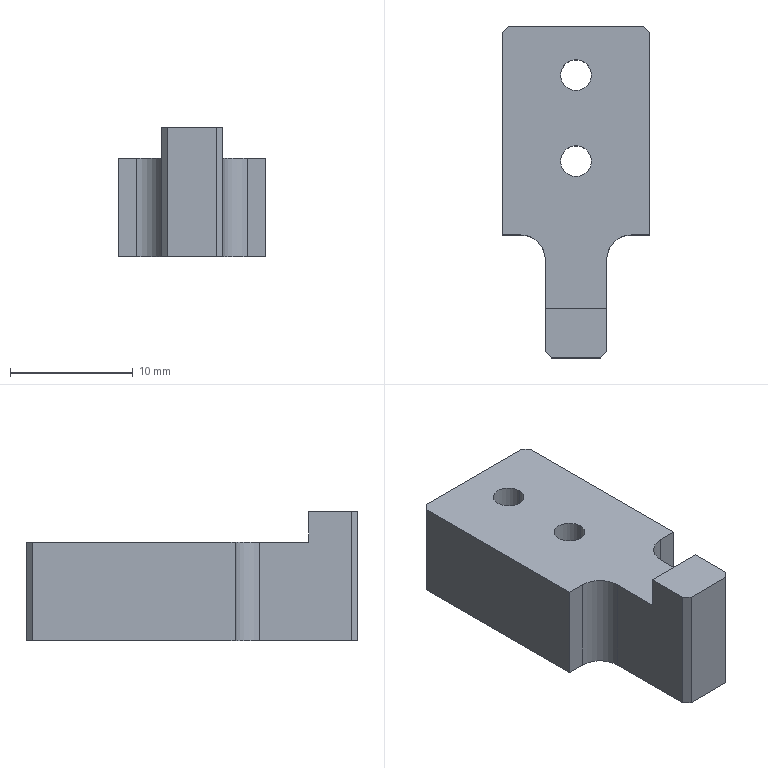Part | SolidWorks | features ICE 3, Chamfer 1, Extrusion 1, HoleWzd 1 | 1 solid | 29 faces | box 12 x 27 x 10.5 mm | volume 1656 mm3 | plane 20 | cylinder 9 | commonest cylinder face diameters 2.5 x4 1 x3 4 x2
STEP:
#1=CARTESIAN_POINT('',(1.25,23.,-2.5));
#2=VERTEX_POINT('',#1);
#3=CARTESIAN_POINT('',(-1.25,23.,-2.5));
#4=VERTEX_POINT('',#3);
#5=CARTESIAN_POINT('',(0.,23.,-2.5));
#6=DIRECTION('',(0.,0.,-1.));
#7=DIRECTION('',(-1.,0.,0.));
#8=AXIS2_PLACEMENT_3D('',#5,#6,#7);
#9=CIRCLE('',#8,1.25);
#10=EDGE_CURVE('',#2,#4,#9,.T.);
#11=ORIENTED_EDGE('',*,*,#10,.F.);
#12=CARTESIAN_POINT('',(1.25,23.,-7.3));
#13=VERTEX_POINT('',#12);
#14=CARTESIAN_POINT('',(1.25,23.,-7.3));
#15=DIRECTION('',(0.,0.,-1.));
#16=VECTOR('',#15,1000.);
#17=LINE('',#14,#16);
#18=EDGE_CURVE('',#2,#13,#17,.T.);
#19=ORIENTED_EDGE('',*,*,#18,.T.);
#20=CARTESIAN_POINT('',(-1.25,23.,-7.3));
#21=VERTEX_POINT('',#20);
#22=CARTESIAN_POINT('',(0.,23.,-7.3));
#23=DIRECTION('',(0.,0.,-1.));
#24=DIRECTION('',(-1.,0.,0.));
#25=AXIS2_PLACEMENT_3D('',#22,#23,#24);
#26=CIRCLE('',#25,1.25);
#27=EDGE_CURVE('',#13,#21,#26,.T.);
#28=ORIENTED_EDGE('',*,*,#27,.T.);
#29=CARTESIAN_POINT('',(-1.25,23.,-7.3));
#30=DIRECTION('',(0.,0.,-1.));
#31=VECTOR('',#30,1000.);
#32=LINE('',#29,#31);
#33=EDGE_CURVE('',#4,#21,#32,.T.);
#34=ORIENTED_EDGE('',*,*,#33,.F.);
#35=EDGE_LOOP('',(#11,#19,#28,#34));
#36=FACE_OUTER_BOUND('',#35,.T.);
#37=CARTESIAN_POINT('',(0.,23.,-7.3));
#38=DIRECTION('',(0.,0.,-1.));
#39=DIRECTION('',(-1.,0.,0.));
#40=AXIS2_PLACEMENT_3D('',#37,#38,#39);
#41=CYLINDRICAL_SURFACE('',#40,1.25);
#42=ADVANCED_FACE('',(#36),#41,.F.);
#43=CARTESIAN_POINT('',(1.25,16.,-2.5));
#44=VERTEX_POINT('',#43);
#45=CARTESIAN_POINT('',(-1.25,16.,-2.5));
#46=VERTEX_POINT('',#45);
#47=CARTESIAN_POINT('',(0.,16.,-2.5));
#48=DIRECTION('',(0.,0.,-1.));
#49=DIRECTION('',(-1.,0.,0.));
#50=AXIS2_PLACEMENT_3D('',#47,#48,#49);
#51=CIRCLE('',#50,1.25);
#52=EDGE_CURVE('',#44,#46,#51,.T.);
#53=ORIENTED_EDGE('',*,*,#52,.F.);
#54=CARTESIAN_POINT('',(1.25,16.,-7.3));
#55=VERTEX_POINT('',#54);
#56=CARTESIAN_POINT('',(1.25,16.,-7.3));
#57=DIRECTION('',(0.,0.,-1.));
#58=VECTOR('',#57,1000.);
#59=LINE('',#56,#58);
#60=EDGE_CURVE('',#44,#55,#59,.T.);
#61=ORIENTED_EDGE('',*,*,#60,.T.);
#62=CARTESIAN_POINT('',(-1.25,16.,-7.3));
#63=VERTEX_POINT('',#62);
#64=CARTESIAN_POINT('',(0.,16.,-7.3));
#65=DIRECTION('',(0.,0.,-1.));
#66=DIRECTION('',(-1.,0.,0.));
#67=AXIS2_PLACEMENT_3D('',#64,#65,#66);
#68=CIRCLE('',#67,1.25);
#69=EDGE_CURVE('',#55,#63,#68,.T.);
#70=ORIENTED_EDGE('',*,*,#69,.T.);
#71=CARTESIAN_POINT('',(-1.25,16.,-7.3));
#72=DIRECTION('',(0.,0.,-1.));
#73=VECTOR('',#72,1000.);
#74=LINE('',#71,#73);
#75=EDGE_CURVE('',#46,#63,#74,.T.);
#76=ORIENTED_EDGE('',*,*,#75,.F.);
#77=EDGE_LOOP('',(#53,#61,#70,#76));
#78=FACE_OUTER_BOUND('',#77,.T.);
#79=CARTESIAN_POINT('',(0.,16.,-7.3));
#80=DIRECTION('',(0.,0.,-1.));
#81=DIRECTION('',(-1.,0.,0.));
#82=AXIS2_PLACEMENT_3D('',#79,#80,#81);
#83=CYLINDRICAL_SURFACE('',#82,1.25);
#84=ADVANCED_FACE('',(#78),#83,.F.);
#85=CARTESIAN_POINT('',(-4.,12.5,-7.3));
#86=VERTEX_POINT('',#85);
#87=CARTESIAN_POINT('',(-4.5,12.,-7.3));
#88=VERTEX_POINT('',#87);
#89=CARTESIAN_POINT('',(-4.,12.,-7.3));
#90=DIRECTION('',(0.,0.,1.));
#91=DIRECTION('',(1.,0.,0.));
#92=AXIS2_PLACEMENT_3D('',#89,#90,#91);
#93=CIRCLE('',#92,0.5);
#94=EDGE_CURVE('',#86,#88,#93,.T.);
#95=ORIENTED_EDGE('',*,*,#94,.T.);
#96=CARTESIAN_POINT('',(-4.5,12.,-10.5));
#97=VERTEX_POINT('',#96);
#98=CARTESIAN_POINT('',(-4.5,12.,-7.3));
#99=DIRECTION('',(0.,0.,-1.));
#100=VECTOR('',#99,1000.);
#101=LINE('',#98,#100);
#102=EDGE_CURVE('',#88,#97,#101,.T.);
#103=ORIENTED_EDGE('',*,*,#102,.T.);
#104=CARTESIAN_POINT('',(-4.,12.5,-10.5));
#105=VERTEX_POINT('',#104);
#106=CARTESIAN_POINT('',(-4.,12.,-10.5));
#107=DIRECTION('',(0.,0.,1.));
#108=DIRECTION('',(1.,0.,0.));
#109=AXIS2_PLACEMENT_3D('',#106,#107,#108);
#110=CIRCLE('',#109,0.5);
#111=EDGE_CURVE('',#105,#97,#110,.T.);
#112=ORIENTED_EDGE('',*,*,#111,.F.);
#113=CARTESIAN_POINT('',(-4.,12.5,-7.3));
#114=DIRECTION('',(0.,0.,-1.));
#115=VECTOR('',#114,1000.);
#116=LINE('',#113,#115);
#117=EDGE_CURVE('',#86,#105,#116,.T.);
#118=ORIENTED_EDGE('',*,*,#117,.F.);
#119=EDGE_LOOP('',(#95,#103,#112,#118));
#120=FACE_OUTER_BOUND('',#119,.T.);
#121=CARTESIAN_POINT('',(-4.,12.,-7.3));
#122=DIRECTION('',(0.,0.,-1.));
#123=DIRECTION('',(-1.,0.,0.));
#124=AXIS2_PLACEMENT_3D('',#121,#122,#123);
#125=CYLINDRICAL_SURFACE('',#124,0.5);
#126=ADVANCED_FACE('',(#120),#125,.F.);
#127=CARTESIAN_POINT('',(2.,0.,-10.5));
#128=VERTEX_POINT('',#127);
#129=CARTESIAN_POINT('',(-2.,0.,-10.5));
#130=VERTEX_POINT('',#129);
#131=CARTESIAN_POINT('',(6.,0.,-10.5));
#132=DIRECTION('',(-1.,0.,0.));
#133=VECTOR('',#132,1000.);
#134=LINE('',#131,#133);
#135=EDGE_CURVE('',#128,#130,#134,.T.);
#136=ORIENTED_EDGE('',*,*,#135,.T.);
#137=CARTESIAN_POINT('',(-2.5,0.5,-10.5));
#138=VERTEX_POINT('',#137);
#139=CARTESIAN_POINT('',(-2.5,0.5,-10.5));
#140=DIRECTION('',(-0.7071,0.7071,0.));
#141=VECTOR('',#140,1000.);
#142=LINE('',#139,#141);
#143=EDGE_CURVE('',#130,#138,#142,.T.);
#144=ORIENTED_EDGE('',*,*,#143,.T.);
#145=CARTESIAN_POINT('',(-2.5,8.,-10.5));
#146=VERTEX_POINT('',#145);
#147=CARTESIAN_POINT('',(-2.5,0.,-10.5));
#148=DIRECTION('',(0.,1.,0.));
#149=VECTOR('',#148,1000.);
#150=LINE('',#147,#149);
#151=EDGE_CURVE('',#138,#146,#150,.T.);
#152=ORIENTED_EDGE('',*,*,#151,.T.);
#153=CARTESIAN_POINT('',(-4.5,10.,-10.5));
#154=VERTEX_POINT('',#153);
#155=CARTESIAN_POINT('',(-4.5,8.,-10.5));
#156=DIRECTION('',(0.,0.,1.));
#157=DIRECTION('',(1.,0.,0.));
#158=AXIS2_PLACEMENT_3D('',#155,#156,#157);
#159=CIRCLE('',#158,2.);
#160=EDGE_CURVE('',#146,#154,#159,.T.);
#161=ORIENTED_EDGE('',*,*,#160,.T.);
#162=CARTESIAN_POINT('',(-6.,10.,-10.5));
#163=VERTEX_POINT('',#162);
#164=CARTESIAN_POINT('',(-6.,10.,-10.5));
#165=DIRECTION('',(-1.,0.,0.));
#166=VECTOR('',#165,1000.);
#167=LINE('',#164,#166);
#168=EDGE_CURVE('',#154,#163,#167,.T.);
#169=ORIENTED_EDGE('',*,*,#168,.T.);
#170=CARTESIAN_POINT('',(-6.,26.5,-10.5));
#171=VERTEX_POINT('',#170);
#172=CARTESIAN_POINT('',(-6.,27.,-10.5));
#173=DIRECTION('',(0.,1.,0.));
#174=VECTOR('',#173,1000.);
#175=LINE('',#172,#174);
#176=EDGE_CURVE('',#163,#171,#175,.T.);
#177=ORIENTED_EDGE('',*,*,#176,.T.);
#178=CARTESIAN_POINT('',(-5.5,27.,-10.5));
#179=VERTEX_POINT('',#178);
#180=CARTESIAN_POINT('',(-5.5,27.,-10.5));
#181=DIRECTION('',(0.7071,0.7071,0.));
#182=VECTOR('',#181,1000.);
#183=LINE('',#180,#182);
#184=EDGE_CURVE('',#171,#179,#183,.T.);
#185=ORIENTED_EDGE('',*,*,#184,.T.);
#186=CARTESIAN_POINT('',(-4.,27.,-10.5));
#187=VERTEX_POINT('',#186);
#188=CARTESIAN_POINT('',(6.,27.,-10.5));
#189=DIRECTION('',(-1.,0.,0.));
#190=VECTOR('',#189,1000.);
#191=LINE('',#188,#190);
#192=EDGE_CURVE('',#187,#179,#191,.T.);
#193=ORIENTED_EDGE('',*,*,#192,.F.);
#194=CARTESIAN_POINT('',(-4.,27.,-10.5));
#195=DIRECTION('',(0.,-1.,0.));
#196=VECTOR('',#195,1000.);
#197=LINE('',#194,#196);
#198=EDGE_CURVE('',#187,#105,#197,.T.);
#199=ORIENTED_EDGE('',*,*,#198,.T.);
#200=ORIENTED_EDGE('',*,*,#111,.T.);
#201=CARTESIAN_POINT('',(-3.5,12.,-10.5));
#202=VERTEX_POINT('',#201);
#203=CARTESIAN_POINT('',(-4.,12.,-10.5));
#204=DIRECTION('',(0.,0.,1.));
#205=DIRECTION('',(1.,0.,0.));
#206=AXIS2_PLACEMENT_3D('',#203,#204,#205);
#207=CIRCLE('',#206,0.5);
#208=EDGE_CURVE('',#97,#202,#207,.T.);
#209=ORIENTED_EDGE('',*,*,#208,.T.);
#210=CARTESIAN_POINT('',(3.5,12.,-10.5));
#211=VERTEX_POINT('',#210);
#212=CARTESIAN_POINT('',(-3.5,12.,-10.5));
#213=DIRECTION('',(1.,0.,0.));
#214=VECTOR('',#213,1000.);
#215=LINE('',#212,#214);
#216=EDGE_CURVE('',#202,#211,#215,.T.);
#217=ORIENTED_EDGE('',*,*,#216,.T.);
#218=CARTESIAN_POINT('',(4.,12.5,-10.5));
#219=VERTEX_POINT('',#218);
#220=CARTESIAN_POINT('',(4.,12.,-10.5));
#221=DIRECTION('',(0.,0.,1.));
#222=DIRECTION('',(1.,0.,0.));
#223=AXIS2_PLACEMENT_3D('',#220,#221,#222);
#224=CIRCLE('',#223,0.5);
#225=EDGE_CURVE('',#211,#219,#224,.T.);
#226=ORIENTED_EDGE('',*,*,#225,.T.);
#227=CARTESIAN_POINT('',(4.,27.,-10.5));
#228=VERTEX_POINT('',#227);
#229=CARTESIAN_POINT('',(4.,27.,-10.5));
#230=DIRECTION('',(0.,1.,0.));
#231=VECTOR('',#230,1000.);
#232=LINE('',#229,#231);
#233=EDGE_CURVE('',#219,#228,#232,.T.);
#234=ORIENTED_EDGE('',*,*,#233,.T.);
#235=CARTESIAN_POINT('',(5.5,27.,-10.5));
#236=VERTEX_POINT('',#235);
#237=CARTESIAN_POINT('',(6.,27.,-10.5));
#238=DIRECTION('',(-1.,0.,0.));
#239=VECTOR('',#238,1000.);
#240=LINE('',#237,#239);
#241=EDGE_CURVE('',#236,#228,#240,.T.);
#242=ORIENTED_EDGE('',*,*,#241,.F.);
#243=CARTESIAN_POINT('',(6.,26.5,-10.5));
#244=VERTEX_POINT('',#243);
#245=CARTESIAN_POINT('',(6.,26.5,-10.5));
#246=DIRECTION('',(0.7071,-0.7071,0.));
#247=VECTOR('',#246,1000.);
#248=LINE('',#245,#247);
#249=EDGE_CURVE('',#236,#244,#248,.T.);
#250=ORIENTED_EDGE('',*,*,#249,.T.);
#251=CARTESIAN_POINT('',(6.,10.,-10.5));
#252=VERTEX_POINT('',#251);
#253=CARTESIAN_POINT('',(6.,27.,-10.5));
#254=DIRECTION('',(0.,1.,0.));
#255=VECTOR('',#254,1000.);
#256=LINE('',#253,#255);
#257=EDGE_CURVE('',#252,#244,#256,.T.);
#258=ORIENTED_EDGE('',*,*,#257,.F.);
#259=CARTESIAN_POINT('',(4.5,10.,-10.5));
#260=VERTEX_POINT('',#259);
#261=CARTESIAN_POINT('',(6.,10.,-10.5));
#262=DIRECTION('',(-1.,0.,0.));
#263=VECTOR('',#262,1000.);
#264=LINE('',#261,#263);
#265=EDGE_CURVE('',#252,#260,#264,.T.);
#266=ORIENTED_EDGE('',*,*,#265,.T.);
#267=CARTESIAN_POINT('',(2.5,8.,-10.5));
#268=VERTEX_POINT('',#267);
#269=CARTESIAN_POINT('',(4.5,8.,-10.5));
#270=DIRECTION('',(0.,0.,1.));
#271=DIRECTION('',(1.,0.,0.));
#272=AXIS2_PLACEMENT_3D('',#269,#270,#271);
#273=CIRCLE('',#272,2.);
#274=EDGE_CURVE('',#260,#268,#273,.T.);
#275=ORIENTED_EDGE('',*,*,#274,.T.);
#276=CARTESIAN_POINT('',(2.5,0.5,-10.5));
#277=VERTEX_POINT('',#276);
#278=CARTESIAN_POINT('',(2.5,0.,-10.5));
#279=DIRECTION('',(0.,-1.,0.));
#280=VECTOR('',#279,1000.);
#281=LINE('',#278,#280);
#282=EDGE_CURVE('',#268,#277,#281,.T.);
#283=ORIENTED_EDGE('',*,*,#282,.T.);
#284=CARTESIAN_POINT('',(2.,0.,-10.5));
#285=DIRECTION('',(-0.7071,-0.7071,0.));
#286=VECTOR('',#285,1000.);
#287=LINE('',#284,#286);
#288=EDGE_CURVE('',#277,#128,#287,.T.);
#289=ORIENTED_EDGE('',*,*,#288,.T.);
#290=EDGE_LOOP('',(#136,#144,#152,#161,#169,#177,#185,#193,#199,#200,#209,#217,#226,#234,#242,#250,#258,#266,#275,#283,#289));
#291=FACE_OUTER_BOUND('',#290,.T.);
#292=CARTESIAN_POINT('',(6.,27.,-10.5));
#293=DIRECTION('',(0.,0.,1.));
#294=DIRECTION('',(0.,-1.,0.));
#295=AXIS2_PLACEMENT_3D('',#292,#293,#294);
#296=PLANE('',#295);
#297=ADVANCED_FACE('',(#291),#296,.F.);
#298=ORIENTED_EDGE('',*,*,#192,.T.);
#299=CARTESIAN_POINT('',(-5.5,27.,-2.5));
#300=VERTEX_POINT('',#299);
#301=CARTESIAN_POINT('',(-5.5,27.,-2.5));
#302=DIRECTION('',(0.,0.,1.));
#303=VECTOR('',#302,1000.);
#304=LINE('',#301,#303);
#305=EDGE_CURVE('',#179,#300,#304,.T.);
#306=ORIENTED_EDGE('',*,*,#305,.T.);
#307=CARTESIAN_POINT('',(5.5,27.,-2.5));
#308=VERTEX_POINT('',#307);
#309=CARTESIAN_POINT('',(6.,27.,-2.5));
#310=DIRECTION('',(-1.,0.,0.));
#311=VECTOR('',#310,1000.);
#312=LINE('',#309,#311);
#313=EDGE_CURVE('',#308,#300,#312,.T.);
#314=ORIENTED_EDGE('',*,*,#313,.F.);
#315=CARTESIAN_POINT('',(5.5,27.,-10.5));
#316=DIRECTION('',(0.,0.,-1.));
#317=VECTOR('',#316,1000.);
#318=LINE('',#315,#317);
#319=EDGE_CURVE('',#308,#236,#318,.T.);
#320=ORIENTED_EDGE('',*,*,#319,.T.);
#321=ORIENTED_EDGE('',*,*,#241,.T.);
#322=CARTESIAN_POINT('',(4.,27.,-7.3));
#323=VERTEX_POINT('',#322);
#324=CARTESIAN_POINT('',(4.,27.,-7.3));
#325=DIRECTION('',(0.,0.,-1.));
#326=VECTOR('',#325,1000.);
#327=LINE('',#324,#326);
#328=EDGE_CURVE('',#323,#228,#327,.T.);
#329=ORIENTED_EDGE('',*,*,#328,.F.);
#330=CARTESIAN_POINT('',(-4.,27.,-7.3));
#331=VERTEX_POINT('',#330);
#332=CARTESIAN_POINT('',(-4.,27.,-7.3));
#333=DIRECTION('',(-1.,0.,0.));
#334=VECTOR('',#333,1000.);
#335=LINE('',#332,#334);
#336=EDGE_CURVE('',#323,#331,#335,.T.);
#337=ORIENTED_EDGE('',*,*,#336,.T.);
#338=CARTESIAN_POINT('',(-4.,27.,-7.3));
#339=DIRECTION('',(0.,0.,-1.));
#340=VECTOR('',#339,1000.);
#341=LINE('',#338,#340);
#342=EDGE_CURVE('',#331,#187,#341,.T.);
#343=ORIENTED_EDGE('',*,*,#342,.T.);
#344=EDGE_LOOP('',(#298,#306,#314,#320,#321,#329,#337,#343));
#345=FACE_OUTER_BOUND('',#344,.T.);
#346=CARTESIAN_POINT('',(6.,27.,-2.5));
#347=DIRECTION('',(0.,-1.,0.));
#348=DIRECTION('',(0.,0.,-1.));
#349=AXIS2_PLACEMENT_3D('',#346,#347,#348);
#350=PLANE('',#349);
#351=ADVANCED_FACE('',(#345),#350,.F.);
#352=CARTESIAN_POINT('',(2.5,4.,0.));
#353=VERTEX_POINT('',#352);
#354=CARTESIAN_POINT('',(-2.5,4.,0.));
#355=VERTEX_POINT('',#354);
#356=CARTESIAN_POINT('',(6.,4.,0.));
#357=DIRECTION('',(-1.,0.,0.));
#358=VECTOR('',#357,1000.);
#359=LINE('',#356,#358);
#360=EDGE_CURVE('',#353,#355,#359,.T.);
#361=ORIENTED_EDGE('',*,*,#360,.F.);
#362=CARTESIAN_POINT('',(2.5,4.,-2.5));
#363=VERTEX_POINT('',#362);
#364=CARTESIAN_POINT('',(2.5,4.,-2.5));
#365=DIRECTION('',(0.,0.,-1.));
#366=VECTOR('',#365,1000.);
#367=LINE('',#364,#366);
#368=EDGE_CURVE('',#353,#363,#367,.T.);
#369=ORIENTED_EDGE('',*,*,#368,.T.);
#370=CARTESIAN_POINT('',(-2.5,4.,-2.5));
#371=VERTEX_POINT('',#370);
#372=CARTESIAN_POINT('',(6.,4.,-2.5));
#373=DIRECTION('',(-1.,0.,0.));
#374=VECTOR('',#373,1000.);
#375=LINE('',#372,#374);
#376=EDGE_CURVE('',#363,#371,#375,.T.);
#377=ORIENTED_EDGE('',*,*,#376,.T.);
#378=CARTESIAN_POINT('',(-2.5,4.,-2.5));
#379=DIRECTION('',(0.,0.,1.));
#380=VECTOR('',#379,1000.);
#381=LINE('',#378,#380);
#382=EDGE_CURVE('',#371,#355,#381,.T.);
#383=ORIENTED_EDGE('',*,*,#382,.T.);
#384=EDGE_LOOP('',(#361,#369,#377,#383));
#385=FACE_OUTER_BOUND('',#384,.T.);
#386=CARTESIAN_POINT('',(6.,4.,-2.5));
#387=DIRECTION('',(0.,-1.,0.));
#388=DIRECTION('',(0.,0.,-1.));
#389=AXIS2_PLACEMENT_3D('',#386,#387,#388);
#390=PLANE('',#389);
#391=ADVANCED_FACE('',(#385),#390,.F.);
#392=CARTESIAN_POINT('',(-2.5,0.5,0.));
#393=VERTEX_POINT('',#392);
#394=CARTESIAN_POINT('',(-2.5,0.,0.));
#395=DIRECTION('',(0.,1.,0.));
#396=VECTOR('',#395,1000.);
#397=LINE('',#394,#396);
#398=EDGE_CURVE('',#393,#355,#397,.T.);
#399=ORIENTED_EDGE('',*,*,#398,.F.);
#400=CARTESIAN_POINT('',(-2.,0.,0.));
#401=VERTEX_POINT('',#400);
#402=CARTESIAN_POINT('',(-2.5,0.5,0.));
#403=DIRECTION('',(0.7071,-0.7071,0.));
#404=VECTOR('',#403,1000.);
#405=LINE('',#402,#404);
#406=EDGE_CURVE('',#393,#401,#405,.T.);
#407=ORIENTED_EDGE('',*,*,#406,.T.);
#408=CARTESIAN_POINT('',(2.,0.,0.));
#409=VERTEX_POINT('',#408);
#410=CARTESIAN_POINT('',(6.,0.,0.));
#411=DIRECTION('',(-1.,0.,0.));
#412=VECTOR('',#411,1000.);
#413=LINE('',#410,#412);
#414=EDGE_CURVE('',#409,#401,#413,.T.);
#415=ORIENTED_EDGE('',*,*,#414,.F.);
#416=CARTESIAN_POINT('',(2.5,0.5,0.));
#417=VERTEX_POINT('',#416);
#418=CARTESIAN_POINT('',(2.,0.,0.));
#419=DIRECTION('',(0.7071,0.7071,0.));
#420=VECTOR('',#419,1000.);
#421=LINE('',#418,#420);
#422=EDGE_CURVE('',#409,#417,#421,.T.);
#423=ORIENTED_EDGE('',*,*,#422,.T.);
#424=CARTESIAN_POINT('',(2.5,0.,0.));
#425=DIRECTION('',(0.,-1.,0.));
#426=VECTOR('',#425,1000.);
#427=LINE('',#424,#426);
#428=EDGE_CURVE('',#353,#417,#427,.T.);
#429=ORIENTED_EDGE('',*,*,#428,.F.);
#430=ORIENTED_EDGE('',*,*,#360,.T.);
#431=EDGE_LOOP('',(#399,#407,#415,#423,#429,#430));
#432=FACE_OUTER_BOUND('',#431,.T.);
#433=CARTESIAN_POINT('',(6.,4.,0.));
#434=DIRECTION('',(0.,0.,-1.));
#435=DIRECTION('',(-1.,0.,0.));
#436=AXIS2_PLACEMENT_3D('',#433,#434,#435);
#437=PLANE('',#436);
#438=ADVANCED_FACE('',(#432),#437,.F.);
#439=ORIENTED_EDGE('',*,*,#414,.T.);
#440=CARTESIAN_POINT('',(-2.,0.,-10.5));
#441=DIRECTION('',(0.,0.,-1.));
#442=VECTOR('',#441,1000.);
#443=LINE('',#440,#442);
#444=EDGE_CURVE('',#401,#130,#443,.T.);
#445=ORIENTED_EDGE('',*,*,#444,.T.);
#446=ORIENTED_EDGE('',*,*,#135,.F.);
#447=CARTESIAN_POINT('',(2.,0.,-10.5));
#448=DIRECTION('',(0.,0.,1.));
#449=VECTOR('',#448,1000.);
#450=LINE('',#447,#449);
#451=EDGE_CURVE('',#128,#409,#450,.T.);
#452=ORIENTED_EDGE('',*,*,#451,.T.);
#453=EDGE_LOOP('',(#439,#445,#446,#452));
#454=FACE_OUTER_BOUND('',#453,.T.);
#455=CARTESIAN_POINT('',(6.,0.,-10.5));
#456=DIRECTION('',(0.,1.,0.));
#457=DIRECTION('',(0.,0.,1.));
#458=AXIS2_PLACEMENT_3D('',#455,#456,#457);
#459=PLANE('',#458);
#460=ADVANCED_FACE('',(#454),#459,.F.);
#461=CARTESIAN_POINT('',(0.,23.,-2.5));
#462=DIRECTION('',(0.,0.,-1.));
#463=DIRECTION('',(-1.,0.,0.));
#464=AXIS2_PLACEMENT_3D('',#461,#462,#463);
#465=CIRCLE('',#464,1.25);
#466=EDGE_CURVE('',#4,#2,#465,.T.);
#467=ORIENTED_EDGE('',*,*,#466,.T.);
#468=ORIENTED_EDGE('',*,*,#10,.T.);
#469=EDGE_LOOP('',(#467,#468));
#470=FACE_BOUND('',#469,.T.);
#471=CARTESIAN_POINT('',(0.,16.,-2.5));
#472=DIRECTION('',(0.,0.,-1.));
#473=DIRECTION('',(-1.,0.,0.));
#474=AXIS2_PLACEMENT_3D('',#471,#472,#473);
#475=CIRCLE('',#474,1.25);
#476=EDGE_CURVE('',#46,#44,#475,.T.);
#477=ORIENTED_EDGE('',*,*,#476,.T.);
#478=ORIENTED_EDGE('',*,*,#52,.T.);
#479=EDGE_LOOP('',(#477,#478));
#480=FACE_BOUND('',#479,.T.);
#481=ORIENTED_EDGE('',*,*,#313,.T.);
#482=CARTESIAN_POINT('',(-6.,26.5,-2.5));
#483=VERTEX_POINT('',#482);
#484=CARTESIAN_POINT('',(-5.5,27.,-2.5));
#485=DIRECTION('',(-0.7071,-0.7071,0.));
#486=VECTOR('',#485,1000.);
#487=LINE('',#484,#486);
#488=EDGE_CURVE('',#300,#483,#487,.T.);
#489=ORIENTED_EDGE('',*,*,#488,.T.);
#490=CARTESIAN_POINT('',(-6.,10.,-2.5));
#491=VERTEX_POINT('',#490);
#492=CARTESIAN_POINT('',(-6.,4.,-2.5));
#493=DIRECTION('',(0.,-1.,0.));
#494=VECTOR('',#493,1000.);
#495=LINE('',#492,#494);
#496=EDGE_CURVE('',#483,#491,#495,.T.);
#497=ORIENTED_EDGE('',*,*,#496,.T.);
#498=CARTESIAN_POINT('',(-4.5,10.,-2.5));
#499=VERTEX_POINT('',#498);
#500=CARTESIAN_POINT('',(6.,10.,-2.5));
#501=DIRECTION('',(1.,0.,0.));
#502=VECTOR('',#501,1000.);
#503=LINE('',#500,#502);
#504=EDGE_CURVE('',#491,#499,#503,.T.);
#505=ORIENTED_EDGE('',*,*,#504,.T.);
#506=CARTESIAN_POINT('',(-2.5,8.,-2.5));
#507=VERTEX_POINT('',#506);
#508=CARTESIAN_POINT('',(-4.5,8.,-2.5));
#509=DIRECTION('',(0.,0.,-1.));
#510=DIRECTION('',(-1.,0.,0.));
#511=AXIS2_PLACEMENT_3D('',#508,#509,#510);
#512=CIRCLE('',#511,2.);
#513=EDGE_CURVE('',#499,#507,#512,.T.);
#514=ORIENTED_EDGE('',*,*,#513,.T.);
#515=CARTESIAN_POINT('',(-2.5,4.,-2.5));
#516=DIRECTION('',(0.,-1.,0.));
#517=VECTOR('',#516,1000.);
#518=LINE('',#515,#517);
#519=EDGE_CURVE('',#507,#371,#518,.T.);
#520=ORIENTED_EDGE('',*,*,#519,.T.);
#521=ORIENTED_EDGE('',*,*,#376,.F.);
#522=CARTESIAN_POINT('',(2.5,8.,-2.5));
#523=VERTEX_POINT('',#522);
#524=CARTESIAN_POINT('',(2.5,4.,-2.5));
#525=DIRECTION('',(0.,1.,0.));
#526=VECTOR('',#525,1000.);
#527=LINE('',#524,#526);
#528=EDGE_CURVE('',#363,#523,#527,.T.);
#529=ORIENTED_EDGE('',*,*,#528,.T.);
#530=CARTESIAN_POINT('',(4.5,10.,-2.5));
#531=VERTEX_POINT('',#530);
#532=CARTESIAN_POINT('',(4.5,8.,-2.5));
#533=DIRECTION('',(0.,0.,-1.));
#534=DIRECTION('',(-1.,0.,0.));
#535=AXIS2_PLACEMENT_3D('',#532,#533,#534);
#536=CIRCLE('',#535,2.);
#537=EDGE_CURVE('',#523,#531,#536,.T.);
#538=ORIENTED_EDGE('',*,*,#537,.T.);
#539=CARTESIAN_POINT('',(6.,10.,-2.5));
#540=VERTEX_POINT('',#539);
#541=CARTESIAN_POINT('',(6.,10.,-2.5));
#542=DIRECTION('',(1.,0.,0.));
#543=VECTOR('',#542,1000.);
#544=LINE('',#541,#543);
#545=EDGE_CURVE('',#531,#540,#544,.T.);
#546=ORIENTED_EDGE('',*,*,#545,.T.);
#547=CARTESIAN_POINT('',(6.,26.5,-2.5));
#548=VERTEX_POINT('',#547);
#549=CARTESIAN_POINT('',(6.,4.,-2.5));
#550=DIRECTION('',(0.,-1.,0.));
#551=VECTOR('',#550,1000.);
#552=LINE('',#549,#551);
#553=EDGE_CURVE('',#548,#540,#552,.T.);
#554=ORIENTED_EDGE('',*,*,#553,.F.);
#555=CARTESIAN_POINT('',(6.,26.5,-2.5));
#556=DIRECTION('',(-0.7071,0.7071,0.));
#557=VECTOR('',#556,1000.);
#558=LINE('',#555,#557);
#559=EDGE_CURVE('',#548,#308,#558,.T.);
#560=ORIENTED_EDGE('',*,*,#559,.T.);
#561=EDGE_LOOP('',(#481,#489,#497,#505,#514,#520,#521,#529,#538,#546,#554,#560));
#562=FACE_OUTER_BOUND('',#561,.T.);
#563=CARTESIAN_POINT('',(6.,4.,-2.5));
#564=DIRECTION('',(0.,0.,-1.));
#565=DIRECTION('',(-1.,0.,0.));
#566=AXIS2_PLACEMENT_3D('',#563,#564,#565);
#567=PLANE('',#566);
#568=ADVANCED_FACE('',(#470,#480,#562),#567,.F.);
#569=ORIENTED_EDGE('',*,*,#257,.T.);
#570=CARTESIAN_POINT('',(6.,26.5,-2.5));
#571=DIRECTION('',(0.,0.,1.));
#572=VECTOR('',#571,1000.);
#573=LINE('',#570,#572);
#574=EDGE_CURVE('',#244,#548,#573,.T.);
#575=ORIENTED_EDGE('',*,*,#574,.T.);
#576=ORIENTED_EDGE('',*,*,#553,.T.);
#577=CARTESIAN_POINT('',(6.,10.,-10.5));
#578=DIRECTION('',(0.,0.,1.));
#579=VECTOR('',#578,1000.);
#580=LINE('',#577,#579);
#581=EDGE_CURVE('',#252,#540,#580,.T.);
#582=ORIENTED_EDGE('',*,*,#581,.F.);
#583=EDGE_LOOP('',(#569,#575,#576,#582));
#584=FACE_OUTER_BOUND('',#583,.T.);
#585=CARTESIAN_POINT('',(6.,0.,0.));
#586=DIRECTION('',(1.,0.,0.));
#587=DIRECTION('',(0.,0.,-1.));
#588=AXIS2_PLACEMENT_3D('',#585,#586,#587);
#589=PLANE('',#588);
#590=ADVANCED_FACE('',(#584),#589,.T.);
#591=ORIENTED_EDGE('',*,*,#496,.F.);
#592=CARTESIAN_POINT('',(-6.,26.5,0.));
#593=DIRECTION('',(0.,0.,-1.));
#594=VECTOR('',#593,1000.);
#595=LINE('',#592,#594);
#596=EDGE_CURVE('',#483,#171,#595,.T.);
#597=ORIENTED_EDGE('',*,*,#596,.T.);
#598=ORIENTED_EDGE('',*,*,#176,.F.);
#599=CARTESIAN_POINT('',(-6.,10.,-10.5));
#600=DIRECTION('',(0.,0.,1.));
#601=VECTOR('',#600,1000.);
#602=LINE('',#599,#601);
#603=EDGE_CURVE('',#163,#491,#602,.T.);
#604=ORIENTED_EDGE('',*,*,#603,.T.);
#605=EDGE_LOOP('',(#591,#597,#598,#604));
#606=FACE_OUTER_BOUND('',#605,.T.);
#607=CARTESIAN_POINT('',(-6.,0.,0.));
#608=DIRECTION('',(1.,0.,0.));
#609=DIRECTION('',(0.,0.,-1.));
#610=AXIS2_PLACEMENT_3D('',#607,#608,#609);
#611=PLANE('',#610);
#612=ADVANCED_FACE('',(#606),#611,.F.);
#613=ORIENTED_EDGE('',*,*,#198,.F.);
#614=ORIENTED_EDGE('',*,*,#342,.F.);
#615=CARTESIAN_POINT('',(-4.,27.,-7.3));
#616=DIRECTION('',(0.,-1.,0.));
#617=VECTOR('',#616,1000.);
#618=LINE('',#615,#617);
#619=EDGE_CURVE('',#331,#86,#618,.T.);
#620=ORIENTED_EDGE('',*,*,#619,.T.);
#621=ORIENTED_EDGE('',*,*,#117,.T.);
#622=EDGE_LOOP('',(#613,#614,#620,#621));
#623=FACE_OUTER_BOUND('',#622,.T.);
#624=CARTESIAN_POINT('',(-4.,27.,-7.3));
#625=DIRECTION('',(1.,0.,0.));
#626=DIRECTION('',(0.,1.,0.));
#627=AXIS2_PLACEMENT_3D('',#624,#625,#626);
#628=PLANE('',#627);
#629=ADVANCED_FACE('',(#623),#628,.T.);
#630=ORIENTED_EDGE('',*,*,#102,.F.);
#631=CARTESIAN_POINT('',(-3.5,12.,-7.3));
#632=VERTEX_POINT('',#631);
#633=CARTESIAN_POINT('',(-4.,12.,-7.3));
#634=DIRECTION('',(0.,0.,1.));
#635=DIRECTION('',(1.,0.,0.));
#636=AXIS2_PLACEMENT_3D('',#633,#634,#635);
#637=CIRCLE('',#636,0.5);
#638=EDGE_CURVE('',#88,#632,#637,.T.);
#639=ORIENTED_EDGE('',*,*,#638,.T.);
#640=CARTESIAN_POINT('',(-3.5,12.,-7.3));
#641=DIRECTION('',(0.,0.,-1.));
#642=VECTOR('',#641,1000.);
#643=LINE('',#640,#642);
#644=EDGE_CURVE('',#632,#202,#643,.T.);
#645=ORIENTED_EDGE('',*,*,#644,.T.);
#646=ORIENTED_EDGE('',*,*,#208,.F.);
#647=EDGE_LOOP('',(#630,#639,#645,#646));
#648=FACE_OUTER_BOUND('',#647,.T.);
#649=CARTESIAN_POINT('',(-4.,12.,-7.3));
#650=DIRECTION('',(0.,0.,-1.));
#651=DIRECTION('',(-1.,0.,0.));
#652=AXIS2_PLACEMENT_3D('',#649,#650,#651);
#653=CYLINDRICAL_SURFACE('',#652,0.5);
#654=ADVANCED_FACE('',(#648),#653,.F.);
#655=ORIENTED_EDGE('',*,*,#216,.F.);
#656=ORIENTED_EDGE('',*,*,#644,.F.);
#657=CARTESIAN_POINT('',(3.5,12.,-7.3));
#658=VERTEX_POINT('',#657);
#659=CARTESIAN_POINT('',(-3.5,12.,-7.3));
#660=DIRECTION('',(1.,0.,0.));
#661=VECTOR('',#660,1000.);
#662=LINE('',#659,#661);
#663=EDGE_CURVE('',#632,#658,#662,.T.);
#664=ORIENTED_EDGE('',*,*,#663,.T.);
#665=CARTESIAN_POINT('',(3.5,12.,-7.3));
#666=DIRECTION('',(0.,0.,-1.));
#667=VECTOR('',#666,1000.);
#668=LINE('',#665,#667);
#669=EDGE_CURVE('',#658,#211,#668,.T.);
#670=ORIENTED_EDGE('',*,*,#669,.T.);
#671=EDGE_LOOP('',(#655,#656,#664,#670));
#672=FACE_OUTER_BOUND('',#671,.T.);
#673=CARTESIAN_POINT('',(-3.5,12.,-7.3));
#674=DIRECTION('',(0.,1.,0.));
#675=DIRECTION('',(0.,0.,1.));
#676=AXIS2_PLACEMENT_3D('',#673,#674,#675);
#677=PLANE('',#676);
#678=ADVANCED_FACE('',(#672),#677,.T.);
#679=ORIENTED_EDGE('',*,*,#225,.F.);
#680=ORIENTED_EDGE('',*,*,#669,.F.);
#681=CARTESIAN_POINT('',(4.,12.5,-7.3));
#682=VERTEX_POINT('',#681);
#683=CARTESIAN_POINT('',(4.,12.,-7.3));
#684=DIRECTION('',(0.,0.,1.));
#685=DIRECTION('',(1.,0.,0.));
#686=AXIS2_PLACEMENT_3D('',#683,#684,#685);
#687=CIRCLE('',#686,0.5);
#688=EDGE_CURVE('',#658,#682,#687,.T.);
#689=ORIENTED_EDGE('',*,*,#688,.T.);
#690=CARTESIAN_POINT('',(4.,12.5,-7.3));
#691=DIRECTION('',(0.,0.,-1.));
#692=VECTOR('',#691,1000.);
#693=LINE('',#690,#692);
#694=EDGE_CURVE('',#682,#219,#693,.T.);
#695=ORIENTED_EDGE('',*,*,#694,.T.);
#696=EDGE_LOOP('',(#679,#680,#689,#695));
#697=FACE_OUTER_BOUND('',#696,.T.);
#698=CARTESIAN_POINT('',(4.,12.,-7.3));
#699=DIRECTION('',(0.,0.,-1.));
#700=DIRECTION('',(-1.,0.,0.));
#701=AXIS2_PLACEMENT_3D('',#698,#699,#700);
#702=CYLINDRICAL_SURFACE('',#701,0.5);
#703=ADVANCED_FACE('',(#697),#702,.F.);
#704=ORIENTED_EDGE('',*,*,#233,.F.);
#705=ORIENTED_EDGE('',*,*,#694,.F.);
#706=CARTESIAN_POINT('',(4.,27.,-7.3));
#707=DIRECTION('',(0.,1.,0.));
#708=VECTOR('',#707,1000.);
#709=LINE('',#706,#708);
#710=EDGE_CURVE('',#682,#323,#709,.T.);
#711=ORIENTED_EDGE('',*,*,#710,.T.);
#712=ORIENTED_EDGE('',*,*,#328,.T.);
#713=EDGE_LOOP('',(#704,#705,#711,#712));
#714=FACE_OUTER_BOUND('',#713,.T.);
#715=CARTESIAN_POINT('',(4.,27.,-7.3));
#716=DIRECTION('',(-1.,0.,0.));
#717=DIRECTION('',(0.,-1.,0.));
#718=AXIS2_PLACEMENT_3D('',#715,#716,#717);
#719=PLANE('',#718);
#720=ADVANCED_FACE('',(#714),#719,.T.);
#721=CARTESIAN_POINT('',(0.,23.,-7.3));
#722=DIRECTION('',(0.,0.,-1.));
#723=DIRECTION('',(-1.,0.,0.));
#724=AXIS2_PLACEMENT_3D('',#721,#722,#723);
#725=CIRCLE('',#724,1.25);
#726=EDGE_CURVE('',#21,#13,#725,.T.);
#727=ORIENTED_EDGE('',*,*,#726,.F.);
#728=ORIENTED_EDGE('',*,*,#27,.F.);
#729=EDGE_LOOP('',(#727,#728));
#730=FACE_BOUND('',#729,.T.);
#731=CARTESIAN_POINT('',(0.,16.,-7.3));
#732=DIRECTION('',(0.,0.,-1.));
#733=DIRECTION('',(-1.,0.,0.));
#734=AXIS2_PLACEMENT_3D('',#731,#732,#733);
#735=CIRCLE('',#734,1.25);
#736=EDGE_CURVE('',#63,#55,#735,.T.);
#737=ORIENTED_EDGE('',*,*,#736,.F.);
#738=ORIENTED_EDGE('',*,*,#69,.F.);
#739=EDGE_LOOP('',(#737,#738));
#740=FACE_BOUND('',#739,.T.);
#741=ORIENTED_EDGE('',*,*,#619,.F.);
#742=ORIENTED_EDGE('',*,*,#336,.F.);
#743=ORIENTED_EDGE('',*,*,#710,.F.);
#744=ORIENTED_EDGE('',*,*,#688,.F.);
#745=ORIENTED_EDGE('',*,*,#663,.F.);
#746=ORIENTED_EDGE('',*,*,#638,.F.);
#747=ORIENTED_EDGE('',*,*,#94,.F.);
#748=EDGE_LOOP('',(#741,#742,#743,#744,#745,#746,#747));
#749=FACE_OUTER_BOUND('',#748,.T.);
#750=CARTESIAN_POINT('',(-4.,12.,-7.3));
#751=DIRECTION('',(0.,0.,1.));
#752=DIRECTION('',(1.,0.,0.));
#753=AXIS2_PLACEMENT_3D('',#750,#751,#752);
#754=PLANE('',#753);
#755=ADVANCED_FACE('',(#730,#740,#749),#754,.F.);
#756=ORIENTED_EDGE('',*,*,#60,.F.);
#757=ORIENTED_EDGE('',*,*,#476,.F.);
#758=ORIENTED_EDGE('',*,*,#75,.T.);
#759=ORIENTED_EDGE('',*,*,#736,.T.);
#760=EDGE_LOOP('',(#756,#757,#758,#759));
#761=FACE_OUTER_BOUND('',#760,.T.);
#762=CARTESIAN_POINT('',(0.,16.,-7.3));
#763=DIRECTION('',(0.,0.,-1.));
#764=DIRECTION('',(-1.,0.,0.));
#765=AXIS2_PLACEMENT_3D('',#762,#763,#764);
#766=CYLINDRICAL_SURFACE('',#765,1.25);
#767=ADVANCED_FACE('',(#761),#766,.F.);
#768=ORIENTED_EDGE('',*,*,#18,.F.);
#769=ORIENTED_EDGE('',*,*,#466,.F.);
#770=ORIENTED_EDGE('',*,*,#33,.T.);
#771=ORIENTED_EDGE('',*,*,#726,.T.);
#772=EDGE_LOOP('',(#768,#769,#770,#771));
#773=FACE_OUTER_BOUND('',#772,.T.);
#774=CARTESIAN_POINT('',(0.,23.,-7.3));
#775=DIRECTION('',(0.,0.,-1.));
#776=DIRECTION('',(-1.,0.,0.));
#777=AXIS2_PLACEMENT_3D('',#774,#775,#776);
#778=CYLINDRICAL_SURFACE('',#777,1.25);
#779=ADVANCED_FACE('',(#773),#778,.F.);
#780=CARTESIAN_POINT('',(-4.5,10.,-10.5));
#781=DIRECTION('',(0.,0.,1.));
#782=VECTOR('',#781,1000.);
#783=LINE('',#780,#782);
#784=EDGE_CURVE('',#154,#499,#783,.T.);
#785=ORIENTED_EDGE('',*,*,#784,.F.);
#786=ORIENTED_EDGE('',*,*,#160,.F.);
#787=CARTESIAN_POINT('',(-2.5,8.,-10.5));
#788=DIRECTION('',(0.,0.,1.));
#789=VECTOR('',#788,1000.);
#790=LINE('',#787,#789);
#791=EDGE_CURVE('',#146,#507,#790,.T.);
#792=ORIENTED_EDGE('',*,*,#791,.T.);
#793=ORIENTED_EDGE('',*,*,#513,.F.);
#794=EDGE_LOOP('',(#785,#786,#792,#793));
#795=FACE_OUTER_BOUND('',#794,.T.);
#796=CARTESIAN_POINT('',(-4.5,8.,-10.5));
#797=DIRECTION('',(0.,0.,1.));
#798=DIRECTION('',(1.,0.,0.));
#799=AXIS2_PLACEMENT_3D('',#796,#797,#798);
#800=CYLINDRICAL_SURFACE('',#799,2.);
#801=ADVANCED_FACE('',(#795),#800,.F.);
#802=ORIENTED_EDGE('',*,*,#151,.F.);
#803=CARTESIAN_POINT('',(-2.5,0.5,-10.5));
#804=DIRECTION('',(0.,0.,1.));
#805=VECTOR('',#804,1000.);
#806=LINE('',#803,#805);
#807=EDGE_CURVE('',#138,#393,#806,.T.);
#808=ORIENTED_EDGE('',*,*,#807,.T.);
#809=ORIENTED_EDGE('',*,*,#398,.T.);
#810=ORIENTED_EDGE('',*,*,#382,.F.);
#811=ORIENTED_EDGE('',*,*,#519,.F.);
#812=ORIENTED_EDGE('',*,*,#791,.F.);
#813=EDGE_LOOP('',(#802,#808,#809,#810,#811,#812));
#814=FACE_OUTER_BOUND('',#813,.T.);
#815=CARTESIAN_POINT('',(-2.5,0.,-10.5));
#816=DIRECTION('',(1.,0.,0.));
#817=DIRECTION('',(0.,1.,0.));
#818=AXIS2_PLACEMENT_3D('',#815,#816,#817);
#819=PLANE('',#818);
#820=ADVANCED_FACE('',(#814),#819,.F.);
#821=ORIENTED_EDGE('',*,*,#603,.F.);
#822=ORIENTED_EDGE('',*,*,#168,.F.);
#823=ORIENTED_EDGE('',*,*,#784,.T.);
#824=ORIENTED_EDGE('',*,*,#504,.F.);
#825=EDGE_LOOP('',(#821,#822,#823,#824));
#826=FACE_OUTER_BOUND('',#825,.T.);
#827=CARTESIAN_POINT('',(-6.,10.,-10.5));
#828=DIRECTION('',(0.,1.,0.));
#829=DIRECTION('',(-1.,0.,0.));
#830=AXIS2_PLACEMENT_3D('',#827,#828,#829);
#831=PLANE('',#830);
#832=ADVANCED_FACE('',(#826),#831,.F.);
#833=ORIENTED_EDGE('',*,*,#428,.T.);
#834=CARTESIAN_POINT('',(2.5,0.5,-10.5));
#835=DIRECTION('',(0.,0.,-1.));
#836=VECTOR('',#835,1000.);
#837=LINE('',#834,#836);
#838=EDGE_CURVE('',#417,#277,#837,.T.);
#839=ORIENTED_EDGE('',*,*,#838,.T.);
#840=ORIENTED_EDGE('',*,*,#282,.F.);
#841=CARTESIAN_POINT('',(2.5,8.,-10.5));
#842=DIRECTION('',(0.,0.,1.));
#843=VECTOR('',#842,1000.);
#844=LINE('',#841,#843);
#845=EDGE_CURVE('',#268,#523,#844,.T.);
#846=ORIENTED_EDGE('',*,*,#845,.T.);
#847=ORIENTED_EDGE('',*,*,#528,.F.);
#848=ORIENTED_EDGE('',*,*,#368,.F.);
#849=EDGE_LOOP('',(#833,#839,#840,#846,#847,#848));
#850=FACE_OUTER_BOUND('',#849,.T.);
#851=CARTESIAN_POINT('',(2.5,0.,-10.5));
#852=DIRECTION('',(-1.,0.,0.));
#853=DIRECTION('',(0.,-1.,0.));
#854=AXIS2_PLACEMENT_3D('',#851,#852,#853);
#855=PLANE('',#854);
#856=ADVANCED_FACE('',(#850),#855,.F.);
#857=ORIENTED_EDGE('',*,*,#845,.F.);
#858=ORIENTED_EDGE('',*,*,#274,.F.);
#859=CARTESIAN_POINT('',(4.5,10.,-10.5));
#860=DIRECTION('',(0.,0.,1.));
#861=VECTOR('',#860,1000.);
#862=LINE('',#859,#861);
#863=EDGE_CURVE('',#260,#531,#862,.T.);
#864=ORIENTED_EDGE('',*,*,#863,.T.);
#865=ORIENTED_EDGE('',*,*,#537,.F.);
#866=EDGE_LOOP('',(#857,#858,#864,#865));
#867=FACE_OUTER_BOUND('',#866,.T.);
#868=CARTESIAN_POINT('',(4.5,8.,-10.5));
#869=DIRECTION('',(0.,0.,1.));
#870=DIRECTION('',(1.,0.,0.));
#871=AXIS2_PLACEMENT_3D('',#868,#869,#870);
#872=CYLINDRICAL_SURFACE('',#871,2.);
#873=ADVANCED_FACE('',(#867),#872,.F.);
#874=ORIENTED_EDGE('',*,*,#863,.F.);
#875=ORIENTED_EDGE('',*,*,#265,.F.);
#876=ORIENTED_EDGE('',*,*,#581,.T.);
#877=ORIENTED_EDGE('',*,*,#545,.F.);
#878=EDGE_LOOP('',(#874,#875,#876,#877));
#879=FACE_OUTER_BOUND('',#878,.T.);
#880=CARTESIAN_POINT('',(6.,10.,-10.5));
#881=DIRECTION('',(0.,1.,0.));
#882=DIRECTION('',(-1.,0.,0.));
#883=AXIS2_PLACEMENT_3D('',#880,#881,#882);
#884=PLANE('',#883);
#885=ADVANCED_FACE('',(#879),#884,.F.);
#886=ORIENTED_EDGE('',*,*,#143,.F.);
#887=ORIENTED_EDGE('',*,*,#444,.F.);
#888=ORIENTED_EDGE('',*,*,#406,.F.);
#889=ORIENTED_EDGE('',*,*,#807,.F.);
#890=EDGE_LOOP('',(#886,#887,#888,#889));
#891=FACE_OUTER_BOUND('',#890,.T.);
#892=CARTESIAN_POINT('',(-2.5,0.5,-10.5));
#893=DIRECTION('',(0.7071,0.7071,0.));
#894=DIRECTION('',(0.,0.,1.));
#895=AXIS2_PLACEMENT_3D('',#892,#893,#894);
#896=PLANE('',#895);
#897=ADVANCED_FACE('',(#891),#896,.F.);
#898=ORIENTED_EDGE('',*,*,#288,.F.);
#899=ORIENTED_EDGE('',*,*,#838,.F.);
#900=ORIENTED_EDGE('',*,*,#422,.F.);
#901=ORIENTED_EDGE('',*,*,#451,.F.);
#902=EDGE_LOOP('',(#898,#899,#900,#901));
#903=FACE_OUTER_BOUND('',#902,.T.);
#904=CARTESIAN_POINT('',(2.,0.,-10.5));
#905=DIRECTION('',(-0.7071,0.7071,0.));
#906=DIRECTION('',(0.,0.,1.));
#907=AXIS2_PLACEMENT_3D('',#904,#905,#906);
#908=PLANE('',#907);
#909=ADVANCED_FACE('',(#903),#908,.F.);
#910=ORIENTED_EDGE('',*,*,#184,.F.);
#911=ORIENTED_EDGE('',*,*,#596,.F.);
#912=ORIENTED_EDGE('',*,*,#488,.F.);
#913=ORIENTED_EDGE('',*,*,#305,.F.);
#914=EDGE_LOOP('',(#910,#911,#912,#913));
#915=FACE_OUTER_BOUND('',#914,.T.);
#916=CARTESIAN_POINT('',(-5.5,27.,-2.5));
#917=DIRECTION('',(0.7071,-0.7071,0.));
#918=DIRECTION('',(0.,0.,1.));
#919=AXIS2_PLACEMENT_3D('',#916,#917,#918);
#920=PLANE('',#919);
#921=ADVANCED_FACE('',(#915),#920,.F.);
#922=ORIENTED_EDGE('',*,*,#249,.F.);
#923=ORIENTED_EDGE('',*,*,#319,.F.);
#924=ORIENTED_EDGE('',*,*,#559,.F.);
#925=ORIENTED_EDGE('',*,*,#574,.F.);
#926=EDGE_LOOP('',(#922,#923,#924,#925));
#927=FACE_OUTER_BOUND('',#926,.T.);
#928=CARTESIAN_POINT('',(6.,26.5,0.));
#929=DIRECTION('',(0.7071,0.7071,0.));
#930=DIRECTION('',(0.,0.,-1.));
#931=AXIS2_PLACEMENT_3D('',#928,#929,#930);
#932=PLANE('',#931);
#933=ADVANCED_FACE('',(#927),#932,.T.);
#934=CLOSED_SHELL('',(#42,#84,#126,#297,#351,#391,#438,#460,#568,#590,#612,#629,#654,#678,#703,#720,#755,#767,#779,#801,#820,#832,#856,#873,#885,#897,#909,#921,#933));
#935=MANIFOLD_SOLID_BREP('',#934);
#936=CARTESIAN_POINT('',(0.,0.,0.));
#937=DIRECTION('',(0.,0.,1.));
#938=DIRECTION('',(1.,0.,0.));
#939=AXIS2_PLACEMENT_3D('',#936,#937,#938);
#940=(LENGTH_UNIT()NAMED_UNIT(*)SI_UNIT(.MILLI.,.METRE.));
#941=UNCERTAINTY_MEASURE_WITH_UNIT(LENGTH_MEASURE(0.00001),#940,'','');
#942=(NAMED_UNIT(*)PLANE_ANGLE_UNIT()SI_UNIT($,.RADIAN.));
#943=(NAMED_UNIT(*)SI_UNIT($,.STERADIAN.)SOLID_ANGLE_UNIT());
#944=(GEOMETRIC_REPRESENTATION_CONTEXT(3)GLOBAL_UNCERTAINTY_ASSIGNED_CONTEXT((#941))GLOBAL_UNIT_ASSIGNED_CONTEXT((#940,#942,#943))REPRESENTATION_CONTEXT('',''));
#945=ADVANCED_BREP_SHAPE_REPRESENTATION('',(#935,#939),#944);